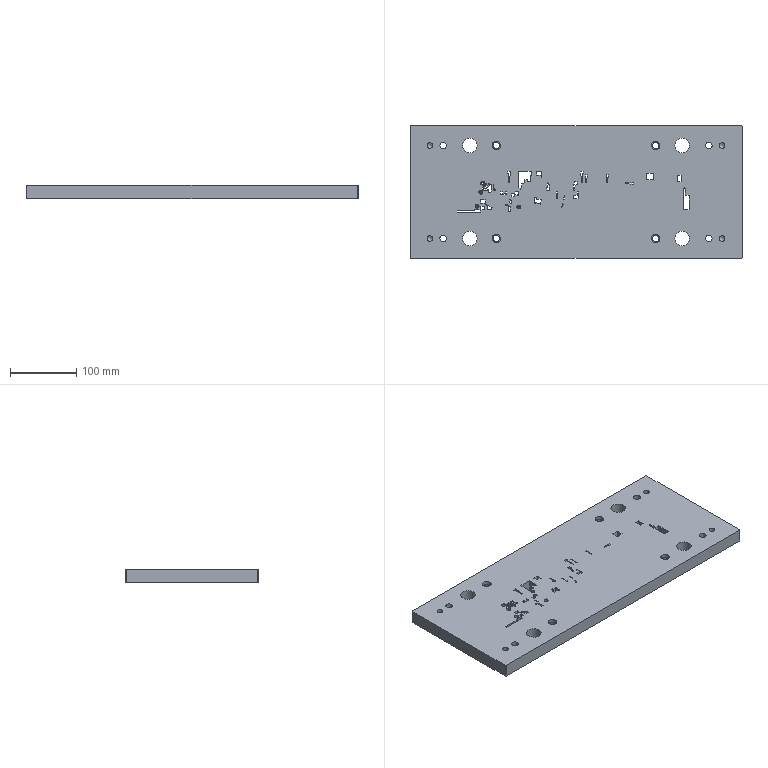Part | NX | features BREP 1 | 1 solid | 391 faces | box 500 x 200 x 20 mm | volume 1921650 mm3 | plane 239 | cylinder 148 | cone 4 | commonest cylinder face diameters 1.05 x65 0.95 x46 10 x8 3 x4 6 x4 8.5 x4